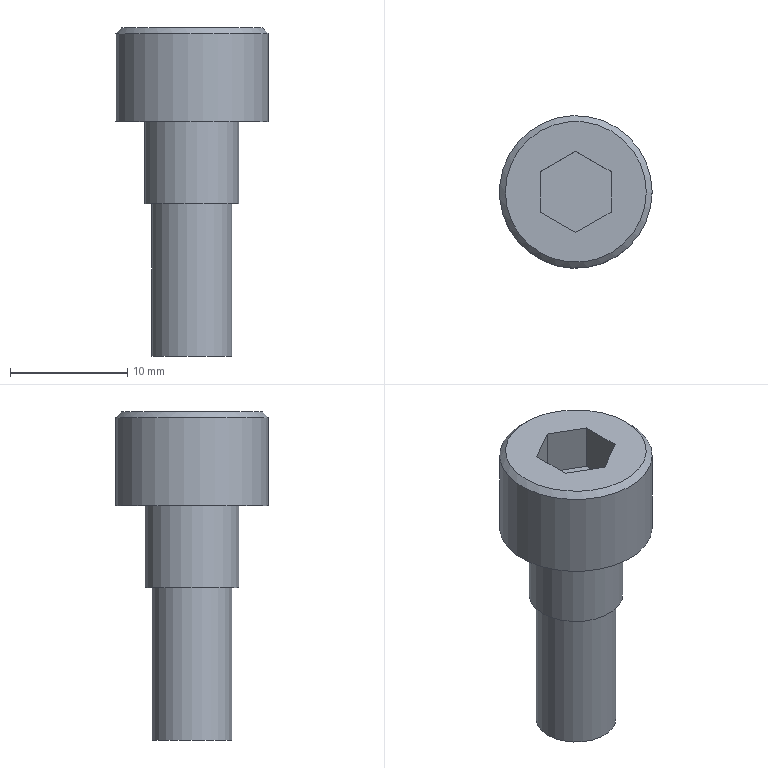Part | STEP file | M3-10_id594_x_t | 1 solid | 15 faces | box 13 x 13 x 28 mm | volume 1756 mm3 | plane 11 | cylinder 3 | cone 1 | commonest cylinder face diameters 6.8 x1 8 x1 13 x1
STEP:
#1=CARTESIAN_POINT('',(-247.4,-170.96,-50.));
#2=VERTEX_POINT('',#1);
#3=CARTESIAN_POINT('',(-244.,-170.96,-50.));
#4=DIRECTION('',(0.,0.,-1.));
#5=DIRECTION('',(-1.,0.,0.));
#6=AXIS2_PLACEMENT_3D('',#3,#4,#5);
#7=CIRCLE('',#6,3.4);
#8=EDGE_CURVE('',#2,#2,#7,.T.);
#9=ORIENTED_EDGE('',*,*,#8,.F.);
#10=EDGE_LOOP('',(#9));
#11=FACE_BOUND('',#10,.T.);
#12=CARTESIAN_POINT('',(-240.,-170.96,-50.));
#13=VERTEX_POINT('',#12);
#14=CARTESIAN_POINT('',(-244.,-170.96,-50.));
#15=DIRECTION('',(0.,0.,1.));
#16=DIRECTION('',(1.,0.,0.));
#17=AXIS2_PLACEMENT_3D('',#14,#15,#16);
#18=CIRCLE('',#17,4.);
#19=EDGE_CURVE('',#13,#13,#18,.T.);
#20=ORIENTED_EDGE('',*,*,#19,.F.);
#21=EDGE_LOOP('',(#20));
#22=FACE_BOUND('',#21,.T.);
#23=CARTESIAN_POINT('',(-244.,-170.96,-50.));
#24=DIRECTION('',(0.,0.,-1.));
#25=DIRECTION('',(-1.,0.,0.));
#26=AXIS2_PLACEMENT_3D('',#23,#24,#25);
#27=PLANE('',#26);
#28=ADVANCED_FACE('',(#11,#22),#27,.T.);
#29=CARTESIAN_POINT('',(-248.,-170.96,-43.));
#30=VERTEX_POINT('',#29);
#31=CARTESIAN_POINT('',(-244.,-170.96,-43.));
#32=DIRECTION('',(0.,0.,1.));
#33=DIRECTION('',(-1.,0.,0.));
#34=AXIS2_PLACEMENT_3D('',#31,#32,#33);
#35=CIRCLE('',#34,4.);
#36=EDGE_CURVE('',#30,#30,#35,.T.);
#37=ORIENTED_EDGE('',*,*,#36,.F.);
#38=EDGE_LOOP('',(#37));
#39=FACE_BOUND('',#38,.T.);
#40=ORIENTED_EDGE('',*,*,#19,.T.);
#41=EDGE_LOOP('',(#40));
#42=FACE_BOUND('',#41,.T.);
#43=CARTESIAN_POINT('',(-244.,-170.96,-50.));
#44=DIRECTION('',(0.,0.,1.));
#45=DIRECTION('',(1.,0.,0.));
#46=AXIS2_PLACEMENT_3D('',#43,#44,#45);
#47=CYLINDRICAL_SURFACE('',#46,4.);
#48=ADVANCED_FACE('',(#39,#42),#47,.T.);
#49=CARTESIAN_POINT('',(-240.6,-170.96,-63.));
#50=VERTEX_POINT('',#49);
#51=CARTESIAN_POINT('',(-244.,-170.96,-63.));
#52=DIRECTION('',(0.,0.,1.));
#53=DIRECTION('',(1.,0.,0.));
#54=AXIS2_PLACEMENT_3D('',#51,#52,#53);
#55=CIRCLE('',#54,3.4);
#56=EDGE_CURVE('',#50,#50,#55,.T.);
#57=ORIENTED_EDGE('',*,*,#56,.F.);
#58=EDGE_LOOP('',(#57));
#59=FACE_OUTER_BOUND('',#58,.T.);
#60=CARTESIAN_POINT('',(-244.,-170.96,-63.));
#61=DIRECTION('',(0.,0.,-1.));
#62=DIRECTION('',(-1.,0.,0.));
#63=AXIS2_PLACEMENT_3D('',#60,#61,#62);
#64=PLANE('',#63);
#65=ADVANCED_FACE('',(#59),#64,.T.);
#66=ORIENTED_EDGE('',*,*,#56,.T.);
#67=EDGE_LOOP('',(#66));
#68=FACE_BOUND('',#67,.T.);
#69=ORIENTED_EDGE('',*,*,#8,.T.);
#70=EDGE_LOOP('',(#69));
#71=FACE_BOUND('',#70,.T.);
#72=CARTESIAN_POINT('',(-244.,-170.96,-50.));
#73=DIRECTION('',(0.,0.,-1.));
#74=DIRECTION('',(1.,0.,0.));
#75=AXIS2_PLACEMENT_3D('',#72,#73,#74);
#76=CYLINDRICAL_SURFACE('',#75,3.4);
#77=ADVANCED_FACE('',(#68,#71),#76,.T.);
#78=CARTESIAN_POINT('',(-247.,-169.228,-35.));
#79=VERTEX_POINT('',#78);
#80=CARTESIAN_POINT('',(-247.,-172.692,-35.));
#81=VERTEX_POINT('',#80);
#82=CARTESIAN_POINT('',(-247.,-169.228,-35.));
#83=DIRECTION('',(0.,-1.,0.));
#84=VECTOR('',#83,1.);
#85=LINE('',#82,#84);
#86=EDGE_CURVE('',#79,#81,#85,.T.);
#87=ORIENTED_EDGE('',*,*,#86,.F.);
#88=CARTESIAN_POINT('',(-244.,-167.496,-35.));
#89=VERTEX_POINT('',#88);
#90=CARTESIAN_POINT('',(-244.,-167.496,-35.));
#91=DIRECTION('',(-0.866,-0.5,0.));
#92=VECTOR('',#91,1.);
#93=LINE('',#90,#92);
#94=EDGE_CURVE('',#89,#79,#93,.T.);
#95=ORIENTED_EDGE('',*,*,#94,.F.);
#96=CARTESIAN_POINT('',(-241.,-169.228,-35.));
#97=VERTEX_POINT('',#96);
#98=CARTESIAN_POINT('',(-241.,-169.228,-35.));
#99=DIRECTION('',(-0.866,0.5,0.));
#100=VECTOR('',#99,1.);
#101=LINE('',#98,#100);
#102=EDGE_CURVE('',#97,#89,#101,.T.);
#103=ORIENTED_EDGE('',*,*,#102,.F.);
#104=CARTESIAN_POINT('',(-241.,-172.692,-35.));
#105=VERTEX_POINT('',#104);
#106=CARTESIAN_POINT('',(-241.,-172.692,-35.));
#107=DIRECTION('',(0.,1.,0.));
#108=VECTOR('',#107,1.);
#109=LINE('',#106,#108);
#110=EDGE_CURVE('',#105,#97,#109,.T.);
#111=ORIENTED_EDGE('',*,*,#110,.F.);
#112=CARTESIAN_POINT('',(-244.,-174.424,-35.));
#113=VERTEX_POINT('',#112);
#114=CARTESIAN_POINT('',(-244.,-174.424,-35.));
#115=DIRECTION('',(0.866,0.5,0.));
#116=VECTOR('',#115,1.);
#117=LINE('',#114,#116);
#118=EDGE_CURVE('',#113,#105,#117,.T.);
#119=ORIENTED_EDGE('',*,*,#118,.F.);
#120=CARTESIAN_POINT('',(-247.,-172.692,-35.));
#121=DIRECTION('',(0.866,-0.5,0.));
#122=VECTOR('',#121,1.);
#123=LINE('',#120,#122);
#124=EDGE_CURVE('',#81,#113,#123,.T.);
#125=ORIENTED_EDGE('',*,*,#124,.F.);
#126=EDGE_LOOP('',(#87,#95,#103,#111,#119,#125));
#127=FACE_BOUND('',#126,.T.);
#128=CARTESIAN_POINT('',(-238.,-170.96,-35.));
#129=VERTEX_POINT('',#128);
#130=CARTESIAN_POINT('',(-244.,-170.96,-35.));
#131=DIRECTION('',(0.,0.,1.));
#132=DIRECTION('',(1.,0.,0.));
#133=AXIS2_PLACEMENT_3D('',#130,#131,#132);
#134=CIRCLE('',#133,6.);
#135=EDGE_CURVE('',#129,#129,#134,.T.);
#136=ORIENTED_EDGE('',*,*,#135,.T.);
#137=EDGE_LOOP('',(#136));
#138=FACE_BOUND('',#137,.T.);
#139=CARTESIAN_POINT('',(-244.,-170.96,-35.));
#140=DIRECTION('',(0.,0.,1.));
#141=DIRECTION('',(1.,0.,0.));
#142=AXIS2_PLACEMENT_3D('',#139,#140,#141);
#143=PLANE('',#142);
#144=ADVANCED_FACE('',(#127,#138),#143,.T.);
#145=ORIENTED_EDGE('',*,*,#36,.T.);
#146=EDGE_LOOP('',(#145));
#147=FACE_BOUND('',#146,.T.);
#148=CARTESIAN_POINT('',(-237.5,-170.96,-43.));
#149=VERTEX_POINT('',#148);
#150=CARTESIAN_POINT('',(-244.,-170.96,-43.));
#151=DIRECTION('',(0.,0.,1.));
#152=DIRECTION('',(1.,0.,0.));
#153=AXIS2_PLACEMENT_3D('',#150,#151,#152);
#154=CIRCLE('',#153,6.5);
#155=EDGE_CURVE('',#149,#149,#154,.T.);
#156=ORIENTED_EDGE('',*,*,#155,.F.);
#157=EDGE_LOOP('',(#156));
#158=FACE_BOUND('',#157,.T.);
#159=CARTESIAN_POINT('',(-244.,-170.96,-43.));
#160=DIRECTION('',(0.,0.,-1.));
#161=DIRECTION('',(-1.,0.,0.));
#162=AXIS2_PLACEMENT_3D('',#159,#160,#161);
#163=PLANE('',#162);
#164=ADVANCED_FACE('',(#147,#158),#163,.T.);
#165=CARTESIAN_POINT('',(-237.5,-170.96,-35.5));
#166=VERTEX_POINT('',#165);
#167=CARTESIAN_POINT('',(-244.,-170.96,-35.5));
#168=DIRECTION('',(0.,0.,-1.));
#169=DIRECTION('',(1.,0.,0.));
#170=AXIS2_PLACEMENT_3D('',#167,#168,#169);
#171=CIRCLE('',#170,6.5);
#172=EDGE_CURVE('',#166,#166,#171,.T.);
#173=ORIENTED_EDGE('',*,*,#172,.T.);
#174=EDGE_LOOP('',(#173));
#175=FACE_BOUND('',#174,.T.);
#176=ORIENTED_EDGE('',*,*,#155,.T.);
#177=EDGE_LOOP('',(#176));
#178=FACE_BOUND('',#177,.T.);
#179=CARTESIAN_POINT('',(-244.,-170.96,-43.));
#180=DIRECTION('',(0.,0.,1.));
#181=DIRECTION('',(1.,0.,0.));
#182=AXIS2_PLACEMENT_3D('',#179,#180,#181);
#183=CYLINDRICAL_SURFACE('',#182,6.5);
#184=ADVANCED_FACE('',(#175,#178),#183,.T.);
#185=ORIENTED_EDGE('',*,*,#135,.F.);
#186=EDGE_LOOP('',(#185));
#187=FACE_BOUND('',#186,.T.);
#188=ORIENTED_EDGE('',*,*,#172,.F.);
#189=EDGE_LOOP('',(#188));
#190=FACE_BOUND('',#189,.T.);
#191=CARTESIAN_POINT('',(-244.,-170.96,-35.5));
#192=DIRECTION('',(0.,0.,-1.));
#193=DIRECTION('',(-1.,0.,0.));
#194=AXIS2_PLACEMENT_3D('',#191,#192,#193);
#195=CONICAL_SURFACE('',#194,6.5,45.);
#196=ADVANCED_FACE('',(#187,#190),#195,.T.);
#197=ORIENTED_EDGE('',*,*,#86,.T.);
#198=CARTESIAN_POINT('',(-247.,-172.692,-39.));
#199=VERTEX_POINT('',#198);
#200=CARTESIAN_POINT('',(-247.,-172.692,-39.));
#201=DIRECTION('',(0.,0.,-1.));
#202=VECTOR('',#201,1.);
#203=LINE('',#200,#202);
#204=EDGE_CURVE('',#81,#199,#203,.T.);
#205=ORIENTED_EDGE('',*,*,#204,.T.);
#206=CARTESIAN_POINT('',(-247.,-169.228,-39.));
#207=VERTEX_POINT('',#206);
#208=CARTESIAN_POINT('',(-247.,-169.228,-39.));
#209=DIRECTION('',(0.,1.,0.));
#210=VECTOR('',#209,1.);
#211=LINE('',#208,#210);
#212=EDGE_CURVE('',#199,#207,#211,.T.);
#213=ORIENTED_EDGE('',*,*,#212,.T.);
#214=CARTESIAN_POINT('',(-247.,-169.228,-39.));
#215=DIRECTION('',(0.,0.,-1.));
#216=VECTOR('',#215,1.);
#217=LINE('',#214,#216);
#218=EDGE_CURVE('',#79,#207,#217,.T.);
#219=ORIENTED_EDGE('',*,*,#218,.F.);
#220=EDGE_LOOP('',(#197,#205,#213,#219));
#221=FACE_OUTER_BOUND('',#220,.T.);
#222=CARTESIAN_POINT('',(-247.,-169.228,-39.));
#223=DIRECTION('',(-1.,0.,0.));
#224=DIRECTION('',(0.,-1.,0.));
#225=AXIS2_PLACEMENT_3D('',#222,#223,#224);
#226=PLANE('',#225);
#227=ADVANCED_FACE('',(#221),#226,.F.);
#228=ORIENTED_EDGE('',*,*,#124,.T.);
#229=CARTESIAN_POINT('',(-244.,-174.424,-39.));
#230=VERTEX_POINT('',#229);
#231=CARTESIAN_POINT('',(-244.,-174.424,-39.));
#232=DIRECTION('',(0.,0.,-1.));
#233=VECTOR('',#232,1.);
#234=LINE('',#231,#233);
#235=EDGE_CURVE('',#113,#230,#234,.T.);
#236=ORIENTED_EDGE('',*,*,#235,.T.);
#237=CARTESIAN_POINT('',(-247.,-172.692,-39.));
#238=DIRECTION('',(-0.866,0.5,0.));
#239=VECTOR('',#238,1.);
#240=LINE('',#237,#239);
#241=EDGE_CURVE('',#230,#199,#240,.T.);
#242=ORIENTED_EDGE('',*,*,#241,.T.);
#243=ORIENTED_EDGE('',*,*,#204,.F.);
#244=EDGE_LOOP('',(#228,#236,#242,#243));
#245=FACE_OUTER_BOUND('',#244,.T.);
#246=CARTESIAN_POINT('',(-247.,-172.692,-39.));
#247=DIRECTION('',(-0.5,-0.866,0.));
#248=DIRECTION('',(0.866,-0.5,0.));
#249=AXIS2_PLACEMENT_3D('',#246,#247,#248);
#250=PLANE('',#249);
#251=ADVANCED_FACE('',(#245),#250,.F.);
#252=ORIENTED_EDGE('',*,*,#118,.T.);
#253=CARTESIAN_POINT('',(-241.,-172.692,-39.));
#254=VERTEX_POINT('',#253);
#255=CARTESIAN_POINT('',(-241.,-172.692,-39.));
#256=DIRECTION('',(0.,0.,-1.));
#257=VECTOR('',#256,1.);
#258=LINE('',#255,#257);
#259=EDGE_CURVE('',#105,#254,#258,.T.);
#260=ORIENTED_EDGE('',*,*,#259,.T.);
#261=CARTESIAN_POINT('',(-244.,-174.424,-39.));
#262=DIRECTION('',(-0.866,-0.5,0.));
#263=VECTOR('',#262,1.);
#264=LINE('',#261,#263);
#265=EDGE_CURVE('',#254,#230,#264,.T.);
#266=ORIENTED_EDGE('',*,*,#265,.T.);
#267=ORIENTED_EDGE('',*,*,#235,.F.);
#268=EDGE_LOOP('',(#252,#260,#266,#267));
#269=FACE_OUTER_BOUND('',#268,.T.);
#270=CARTESIAN_POINT('',(-244.,-174.424,-39.));
#271=DIRECTION('',(0.5,-0.866,0.));
#272=DIRECTION('',(0.866,0.5,0.));
#273=AXIS2_PLACEMENT_3D('',#270,#271,#272);
#274=PLANE('',#273);
#275=ADVANCED_FACE('',(#269),#274,.F.);
#276=ORIENTED_EDGE('',*,*,#110,.T.);
#277=CARTESIAN_POINT('',(-241.,-169.228,-39.));
#278=VERTEX_POINT('',#277);
#279=CARTESIAN_POINT('',(-241.,-169.228,-39.));
#280=DIRECTION('',(0.,0.,-1.));
#281=VECTOR('',#280,1.);
#282=LINE('',#279,#281);
#283=EDGE_CURVE('',#97,#278,#282,.T.);
#284=ORIENTED_EDGE('',*,*,#283,.T.);
#285=CARTESIAN_POINT('',(-241.,-172.692,-39.));
#286=DIRECTION('',(0.,-1.,0.));
#287=VECTOR('',#286,1.);
#288=LINE('',#285,#287);
#289=EDGE_CURVE('',#278,#254,#288,.T.);
#290=ORIENTED_EDGE('',*,*,#289,.T.);
#291=ORIENTED_EDGE('',*,*,#259,.F.);
#292=EDGE_LOOP('',(#276,#284,#290,#291));
#293=FACE_OUTER_BOUND('',#292,.T.);
#294=CARTESIAN_POINT('',(-241.,-172.692,-39.));
#295=DIRECTION('',(1.,0.,0.));
#296=DIRECTION('',(0.,1.,0.));
#297=AXIS2_PLACEMENT_3D('',#294,#295,#296);
#298=PLANE('',#297);
#299=ADVANCED_FACE('',(#293),#298,.F.);
#300=ORIENTED_EDGE('',*,*,#102,.T.);
#301=CARTESIAN_POINT('',(-244.,-167.496,-39.));
#302=VERTEX_POINT('',#301);
#303=CARTESIAN_POINT('',(-244.,-167.496,-39.));
#304=DIRECTION('',(0.,0.,-1.));
#305=VECTOR('',#304,1.);
#306=LINE('',#303,#305);
#307=EDGE_CURVE('',#89,#302,#306,.T.);
#308=ORIENTED_EDGE('',*,*,#307,.T.);
#309=CARTESIAN_POINT('',(-241.,-169.228,-39.));
#310=DIRECTION('',(0.866,-0.5,0.));
#311=VECTOR('',#310,1.);
#312=LINE('',#309,#311);
#313=EDGE_CURVE('',#302,#278,#312,.T.);
#314=ORIENTED_EDGE('',*,*,#313,.T.);
#315=ORIENTED_EDGE('',*,*,#283,.F.);
#316=EDGE_LOOP('',(#300,#308,#314,#315));
#317=FACE_OUTER_BOUND('',#316,.T.);
#318=CARTESIAN_POINT('',(-241.,-169.228,-39.));
#319=DIRECTION('',(0.5,0.866,0.));
#320=DIRECTION('',(-0.866,0.5,0.));
#321=AXIS2_PLACEMENT_3D('',#318,#319,#320);
#322=PLANE('',#321);
#323=ADVANCED_FACE('',(#317),#322,.F.);
#324=ORIENTED_EDGE('',*,*,#94,.T.);
#325=ORIENTED_EDGE('',*,*,#218,.T.);
#326=CARTESIAN_POINT('',(-244.,-167.496,-39.));
#327=DIRECTION('',(0.866,0.5,0.));
#328=VECTOR('',#327,1.);
#329=LINE('',#326,#328);
#330=EDGE_CURVE('',#207,#302,#329,.T.);
#331=ORIENTED_EDGE('',*,*,#330,.T.);
#332=ORIENTED_EDGE('',*,*,#307,.F.);
#333=EDGE_LOOP('',(#324,#325,#331,#332));
#334=FACE_OUTER_BOUND('',#333,.T.);
#335=CARTESIAN_POINT('',(-244.,-167.496,-39.));
#336=DIRECTION('',(-0.5,0.866,0.));
#337=DIRECTION('',(-0.866,-0.5,0.));
#338=AXIS2_PLACEMENT_3D('',#335,#336,#337);
#339=PLANE('',#338);
#340=ADVANCED_FACE('',(#334),#339,.F.);
#341=ORIENTED_EDGE('',*,*,#212,.F.);
#342=ORIENTED_EDGE('',*,*,#241,.F.);
#343=ORIENTED_EDGE('',*,*,#265,.F.);
#344=ORIENTED_EDGE('',*,*,#289,.F.);
#345=ORIENTED_EDGE('',*,*,#313,.F.);
#346=ORIENTED_EDGE('',*,*,#330,.F.);
#347=EDGE_LOOP('',(#341,#342,#343,#344,#345,#346));
#348=FACE_OUTER_BOUND('',#347,.T.);
#349=CARTESIAN_POINT('',(-244.,-170.96,-39.));
#350=DIRECTION('',(0.,0.,1.));
#351=DIRECTION('',(1.,0.,0.));
#352=AXIS2_PLACEMENT_3D('',#349,#350,#351);
#353=PLANE('',#352);
#354=ADVANCED_FACE('',(#348),#353,.T.);
#355=CLOSED_SHELL('',(#28,#48,#65,#77,#144,#164,#184,#196,#227,#251,#275,#299,#323,#340,#354));
#356=MANIFOLD_SOLID_BREP('',#355);
#357=(LENGTH_UNIT()NAMED_UNIT(*)SI_UNIT(.MILLI.,.METRE.));
#358=UNCERTAINTY_MEASURE_WITH_UNIT(LENGTH_MEASURE(0.00002),#357,'','');
#359=(NAMED_UNIT(*)PLANE_ANGLE_UNIT()SI_UNIT($,.RADIAN.));
#360=PLANE_ANGLE_MEASURE_WITH_UNIT(PLANE_ANGLE_MEASURE(0.01745),#359);
#361=DIMENSIONAL_EXPONENTS(0.,0.,0.,0.,0.,0.,0.);
#362=(CONVERSION_BASED_UNIT('DEGREE',#360)NAMED_UNIT(#361)PLANE_ANGLE_UNIT());
#363=(NAMED_UNIT(*)SI_UNIT($,.STERADIAN.)SOLID_ANGLE_UNIT());
#364=(GEOMETRIC_REPRESENTATION_CONTEXT(3)GLOBAL_UNCERTAINTY_ASSIGNED_CONTEXT((#358))GLOBAL_UNIT_ASSIGNED_CONTEXT((#357,#362,#363))REPRESENTATION_CONTEXT('',''));
#365=ADVANCED_BREP_SHAPE_REPRESENTATION('',(#356),#364);